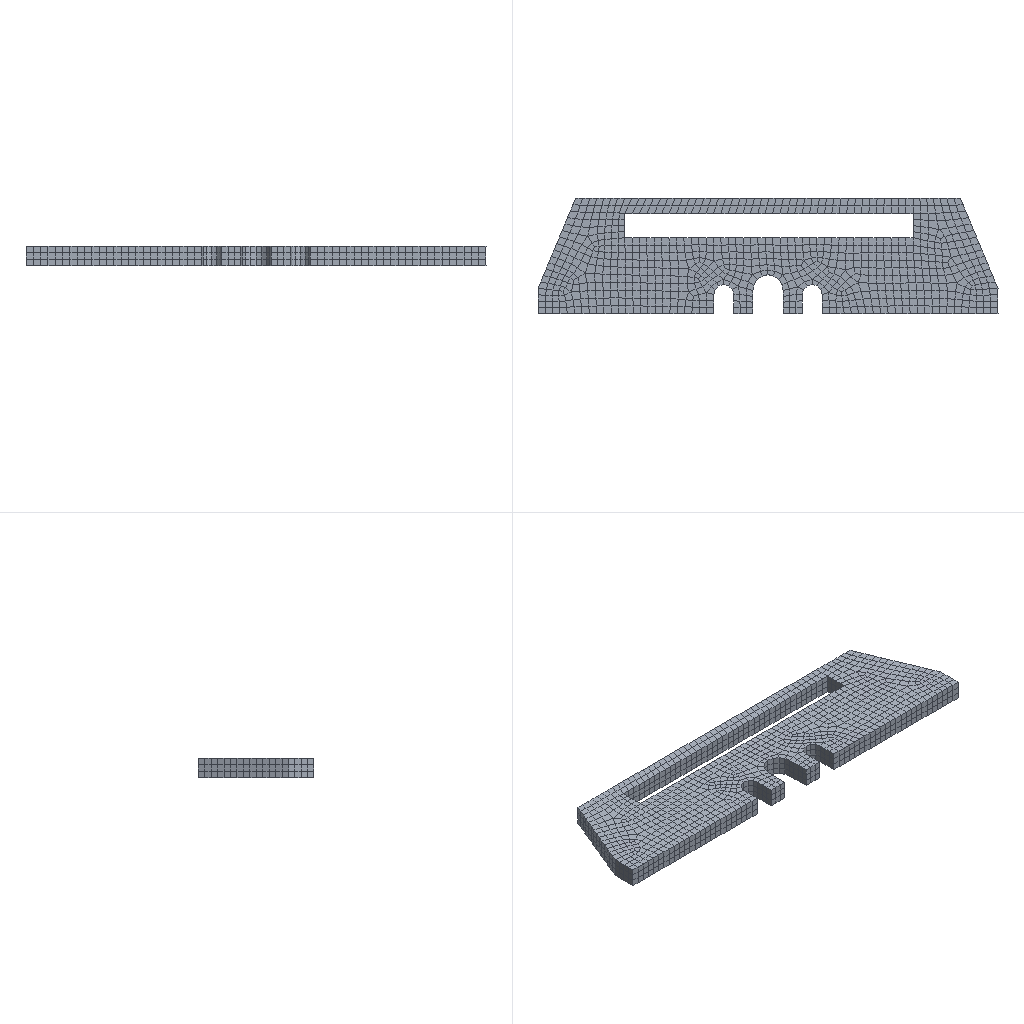Simulation study | ansys workbench
Ansys APDL input file, long lists of numbers shortened:
/batch
/config,noeldb,1     ! force off writing results to database
*get,_wallstrt,active,,time,wall
! ANSYS input file written by Workbench version 17.0 RELEASE
! File used for geometry attach:
/title,The wall thermal analysis--Steady-State Thermal (A5)
*DIM,_wb_ProjectScratch_dir,string,248
_wb_ProjectScratch_dir(1) = ''
*DIM,_wb_SolverFiles_dir,string,248
_wb_SolverFiles_dir(1) = ''
*DIM,_wb_userfiles_dir,string,248
_wb_userfiles_dir(1) = ''
/com,--- Data in consistent NMM units. See Solving Units in the help system for more information.
/units,MPA
/nopr
/wb,file,start              !  signify a WB generated input file
/prep7
! Turn off shape checking because checks already performed inside WB mesher.
! See help system for more information.
SHPP,OFF,,NOWARN
/nolist
etcon,set             ! allow ANSYS to choose best KEYOP's for 180x elements
/com,*********** Nodes for the whole assembly ***********
nblock,3
(1i9,3e20.9e3)
        1    1.298159564E+004    3.180623967E+003    0.000000000E+000
! (13514 more lines like these left out)
-1
/wb,elem,start            !  set before creation of elements
/com,*********** Elements for Body 1 "Wall" ***********
et,1,90
eblock,19,solid,,2406
(19i9)
        1        1        1        1        0        0        0        0       20        0        1     2811     2810     2434     2641     3748     3747     3371     3578
! (4811 more lines like these left out)
-1
/wb,elem,end               !  done creating elements
/com,*********** Send User Defined Coordinate System(s) ***********
csys,0
toffst,273.15,  ! Temperature offset from absolute zero
/wb,mat,start              !  starting to send materials
/com,*********** Send Materials ***********
MP,DENS,1,1.64e-09,	! tonne mm^-3
MP,ALPX,1,5e-06,	! C^-1
MP,C,1,960000000,	! mm^2 s^-2 C^-1
MP,KXX,1,52.78,	! tonne mm s^-3 C^-1
MP,EX,1,2230,	! tonne s^-2 mm^-1
MP,NUXY,1,0.1,
/wb,mat,end                !  done sending materials
!************************* Model Summary ********************
!Wall,	wall,	matid,	1
!************************* End Model Summary ********************
! get the diagonal of the bounding box. Needed later for other things
*get,_xmin,node,,mnloc,x
*get,_ymin,node,,mnloc,y
*get,_zmin,node,,mnloc,z
*get,_xmax,node,,mxloc,x
*get,_ymax,node,,mxloc,y
*get,_zmax,node,,mxloc,z
_ASMDIAG=(_xmax-_xmin)*(_xmax-_xmin)+(_ymax-_ymin)*(_ymax-_ymin)+(_zmax-_zmin)*(_zmax-_zmin)
_ASMDIAG=SQRT(_ASMDIAG)
/wb,contact,start          !  starting to send contact
/wb,contact,end            !  done creating contacts
/golist
/wb,load,start             !  starting to send loads
/com,*********** Define Temperature Constraint ***********
CMBLOCK,_CM29   ,NODE,     2676
(8i10)
         1         2         3         4         9        10        11        15
! (334 more lines like these left out)
*DIM,_loadvari29,TABLE,2,2,1,X,TIME
! Time Values
_loadvari29(0,1,1) = 0.
_loadvari29(0,2,1) = 1.
! X values
_loadvari29(1,0,1) = -23909.
_loadvari29(2,0,1) = 23909.
! Load values
_loadvari29(1,1,1) = 0.
_loadvari29(1,2,1) = -12.
_loadvari29(2,1,1) = 0.
_loadvari29(2,2,1) = -15.
fcum,add                   ! add nodal forces up (needed in case have loads on the same edge,vertex)
fcum                       ! reset default on fcum command since done sending WB F loads
/com,*********** Create "Convection" ***********
et,2,152
eblock,10,,,648
(15i9)
     2407        2        2        2        0     3484     2547     2681     3618    13011    10757     4220     4182
! (647 more lines like these left out)
-1
esel,s,type,,2
keyop,2,8,2.
keyop,2,13,0.
*DIM,_convvari99,TABLE,1,1,1,TEMP,
! Temperature values
_convvari99(1,0,1) = 5.
! Load values
_convvari99(1,1,1) = 5.e-003
*DIM,_loadvari99,TABLE,2,1,1,TIME,
! Time values
_loadvari99(1,0,1) = 0.
_loadvari99(2,0,1) = 1.
! Load values
_loadvari99(1,1,1) = 5.
_loadvari99(2,1,1) = 5.
esel,all
/com,***************** Define Uniform Initial temperature ***************
tunif,5.
/gst,on,on
fini
*get,_numnode,node,0,count
*get,_numelem,elem,0,count
*get, _MAXELEMNUM, elem, 0, NUM, MAX
*get, _MAXNODENUM, node, 0, NUM, MAX
*get, _MAXELEMTYPE, etyp, 0, NUM, MAX
*get, _MAXREALCONST, real, 0, NUM, MAX
/go
/wb,load,end               !  done creating loads
/com,--- Number of total nodes = %_numnode%
/com,--- Number of contact elements = 648
/com,--- Number of spring elements = 0
/com,--- Number of bearing elements = 0
/com,--- Number of solid elements = 2406
/com,--- Number of total elements = %_numelem%
*get,_wallbsol,active,,time,wall
/com,****************************************************************************
/com,*************************    SOLUTION       ********************************
/com,****************************************************************************
/solu
antype,0                   ! static analysis
!eqsl,sparse               ! using sparse solver which is default so no eqsl command needed
cntr,print,1               ! print out contact info and also make no initial contact an error
resc,,none                 ! Do not keep any restart files
rstsuppress,cont           ! Don't write contact results
dmpopt,emat,no             ! Don't combine emat file for DANSYS
dmpopt,esav,no             ! Don't combine esav file for DANSYS
/com,****************************************************
/com,******************* SOLVE FOR LS 1 ****************
d,_CM29,temp,%_loadvari29%
esel,s,type,,2
nsle
sf,all,conv,%_convvari99%,%_loadvari99%
nsel,all
esel,all
autots,on
nsub,1,10,1
time,1.
outres,erase
outres,all,none
outres,nsol,all
outres,rsol,all
outres,fflux,all
/nopr
esel,s,mat,,2
cm,_elmisc,elem
esel,all
/gopr
outres,misc,all,_elmisc
cnvtol,heat,,.001,,1.e-003	! Program Controlled. Set MINREF equivalent of 1e-6 Watts
! *********** WB SOLVE COMMAND ***********
! check interactive state
*get,ANSINTER_,active,,int
*if,ANSINTER_,ne,0,then
/eof
*endif
solve
/com *************** Write FE CONNECTORS *********
CEWRITE,file,ce,,INTE
/com,****************************************************
/com,*************** FINISHED SOLVE FOR LS 1 *************
*set,_DS_PROGRESS          ! turn off progress updates to avoid virus scanning bug
*get,_wallasol,active,,time,wall
/post1
xmlo,ENCODING,ISO-8859-1
xmlo,parm
/xml,parm,xml
fini
/gopr
*get,_walldone,active,,time,wall
_preptime=(_wallbsol-_wallstrt)*3600
_solvtime=(_wallasol-_wallbsol)*3600
_posttime=(_walldone-_wallasol)*3600
_totaltim=(_walldone-_wallstrt)*3600
/wb,file,end               ! done with WB generated input